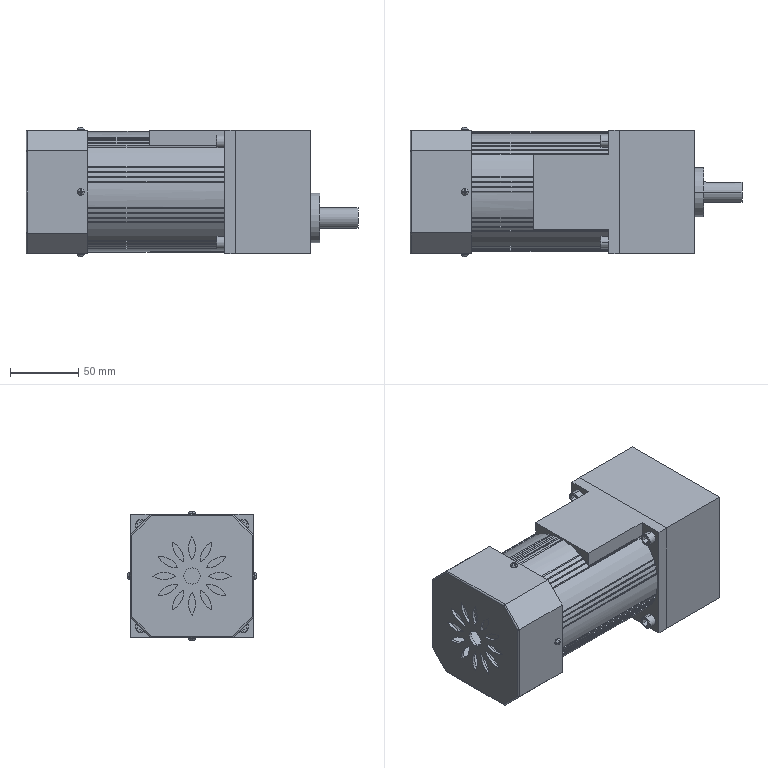Part | SolidWorks | features MBimport 1 | 8 solids | 354 faces | box 242.5 x 94.951 x 94.951 mm | volume 1199171 mm3 | plane 171 | cylinder 159 | sphere 8 | cone 8 | torus 8 | commonest cylinder face diameters 1.5 x44 87 x36 30 x30 5 x17 2 x8 6 x8